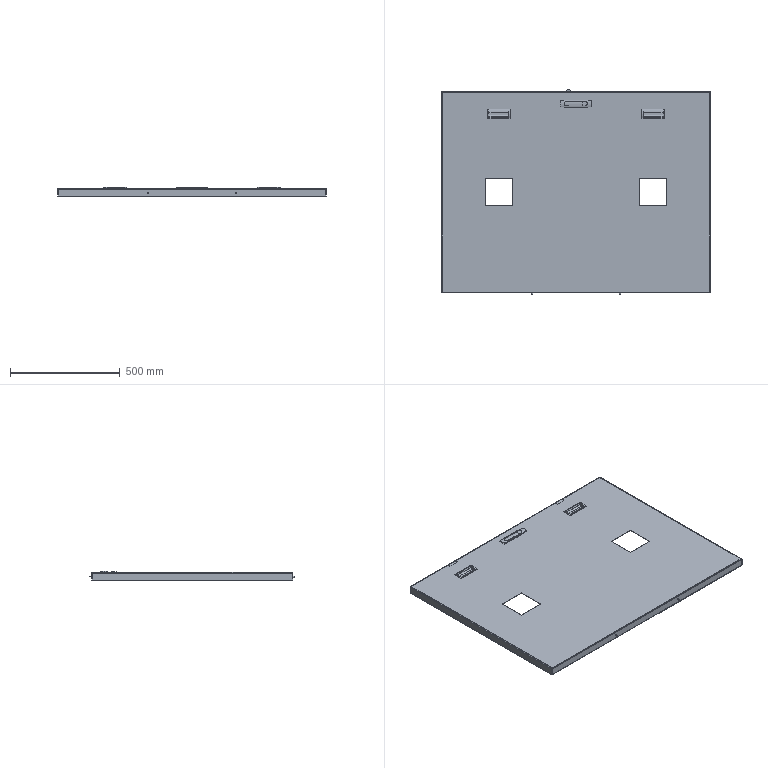Part | SolidWorks | 8 solids | 548 faces | box 1225 x 936.5 x 44 mm | volume 2112957 mm3 | plane 260 | cylinder 210 | spline 46 | cone 26 | torus 6 | commonest cylinder face diameters 10 x27 2 x20 3.3 x16 8.136 x15 7 x13 4 x12